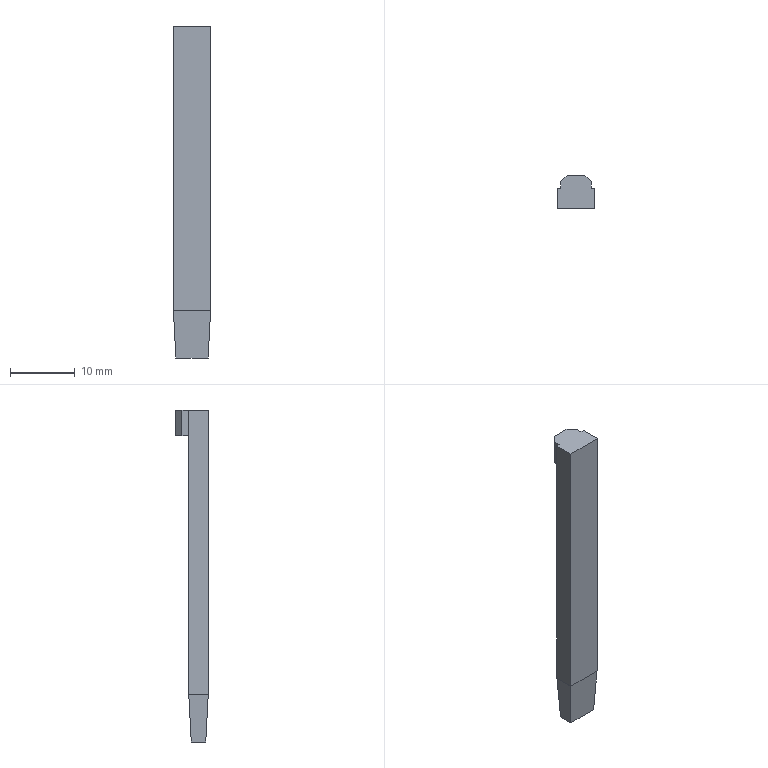Part | Creo | 1 solid | 21 faces | box 5.838 x 5.102 x 51.155 mm | volume 930.54 mm3 | plane 21
STEP:
#1=CARTESIAN_POINT('',(0.,0.,0.));
#2=DIRECTION('',(0.,0.,1.));
#3=DIRECTION('',(1.,0.,0.));
#4=AXIS2_PLACEMENT_3D('',#1,#2,#3);
#5=CARTESIAN_POINT('',(12.137,6.97,42.091));
#6=VERTEX_POINT('',#5);
#7=CARTESIAN_POINT('',(12.137,10.072,42.091));
#8=VERTEX_POINT('',#7);
#9=CARTESIAN_POINT('',(12.137,6.97,42.091));
#10=DIRECTION('',(0.,1.,0.));
#11=VECTOR('',#10,3.102);
#12=LINE('',#9,#11);
#13=EDGE_CURVE('',#6,#8,#12,.T.);
#14=ORIENTED_EDGE('',*,*,#13,.T.);
#15=CARTESIAN_POINT('',(6.299,10.072,42.091));
#16=VERTEX_POINT('',#15);
#17=CARTESIAN_POINT('',(12.137,10.072,42.091));
#18=DIRECTION('',(-1.,0.,0.));
#19=VECTOR('',#18,5.838);
#20=LINE('',#17,#19);
#21=EDGE_CURVE('',#8,#16,#20,.T.);
#22=ORIENTED_EDGE('',*,*,#21,.T.);
#23=CARTESIAN_POINT('',(6.299,6.97,42.091));
#24=VERTEX_POINT('',#23);
#25=CARTESIAN_POINT('',(6.299,10.072,42.091));
#26=DIRECTION('',(0.,-1.,0.));
#27=VECTOR('',#26,3.102);
#28=LINE('',#25,#27);
#29=EDGE_CURVE('',#16,#24,#28,.T.);
#30=ORIENTED_EDGE('',*,*,#29,.T.);
#31=CARTESIAN_POINT('',(6.299,6.97,42.091));
#32=DIRECTION('',(1.,0.,0.));
#33=VECTOR('',#32,5.838);
#34=LINE('',#31,#33);
#35=EDGE_CURVE('',#24,#6,#34,.T.);
#36=ORIENTED_EDGE('',*,*,#35,.T.);
#37=EDGE_LOOP('',(#14,#22,#30,#36));
#38=FACE_OUTER_BOUND('',#37,.F.);
#39=CARTESIAN_POINT('',(12.087,7.02,42.091));
#40=VERTEX_POINT('',#39);
#41=CARTESIAN_POINT('',(12.087,10.022,42.091));
#42=VERTEX_POINT('',#41);
#43=CARTESIAN_POINT('',(12.087,7.02,42.091));
#44=DIRECTION('',(0.,1.,0.));
#45=VECTOR('',#44,3.002);
#46=LINE('',#43,#45);
#47=EDGE_CURVE('',#40,#42,#46,.T.);
#48=ORIENTED_EDGE('',*,*,#47,.F.);
#49=CARTESIAN_POINT('',(6.349,7.02,42.091));
#50=VERTEX_POINT('',#49);
#51=CARTESIAN_POINT('',(6.349,7.02,42.091));
#52=DIRECTION('',(1.,0.,0.));
#53=VECTOR('',#52,5.738);
#54=LINE('',#51,#53);
#55=EDGE_CURVE('',#50,#40,#54,.T.);
#56=ORIENTED_EDGE('',*,*,#55,.F.);
#57=CARTESIAN_POINT('',(6.349,10.022,42.091));
#58=VERTEX_POINT('',#57);
#59=CARTESIAN_POINT('',(6.349,10.022,42.091));
#60=DIRECTION('',(0.,-1.,0.));
#61=VECTOR('',#60,3.002);
#62=LINE('',#59,#61);
#63=EDGE_CURVE('',#58,#50,#62,.T.);
#64=ORIENTED_EDGE('',*,*,#63,.F.);
#65=CARTESIAN_POINT('',(6.349,10.022,42.091));
#66=DIRECTION('',(1.,0.,0.));
#67=VECTOR('',#66,5.738);
#68=LINE('',#65,#67);
#69=EDGE_CURVE('',#58,#42,#68,.T.);
#70=ORIENTED_EDGE('',*,*,#69,.T.);
#71=EDGE_LOOP('',(#48,#56,#64,#70));
#72=FACE_BOUND('',#71,.F.);
#73=CARTESIAN_POINT('',(12.087,10.022,42.091));
#74=DIRECTION('',(0.,0.,1.));
#75=DIRECTION('',(1.,0.,0.));
#76=AXIS2_PLACEMENT_3D('',#73,#74,#75);
#77=PLANE('',#76);
#78=ADVANCED_FACE('',(#38,#72),#77,.F.);
#79=CARTESIAN_POINT('',(12.137,6.97,85.91));
#80=VERTEX_POINT('',#79);
#81=CARTESIAN_POINT('',(12.137,6.97,85.91));
#82=DIRECTION('',(0.,0.,-1.));
#83=VECTOR('',#82,43.819);
#84=LINE('',#81,#83);
#85=EDGE_CURVE('',#80,#6,#84,.T.);
#86=ORIENTED_EDGE('',*,*,#85,.F.);
#87=CARTESIAN_POINT('',(12.137,10.072,85.91));
#88=VERTEX_POINT('',#87);
#89=CARTESIAN_POINT('',(12.137,6.97,85.91));
#90=DIRECTION('',(0.,1.,0.));
#91=VECTOR('',#90,3.102);
#92=LINE('',#89,#91);
#93=EDGE_CURVE('',#80,#88,#92,.T.);
#94=ORIENTED_EDGE('',*,*,#93,.T.);
#95=CARTESIAN_POINT('',(12.137,10.072,85.91));
#96=DIRECTION('',(0.,0.,-1.));
#97=VECTOR('',#96,43.819);
#98=LINE('',#95,#97);
#99=EDGE_CURVE('',#88,#8,#98,.T.);
#100=ORIENTED_EDGE('',*,*,#99,.T.);
#101=ORIENTED_EDGE('',*,*,#13,.F.);
#102=EDGE_LOOP('',(#86,#94,#100,#101));
#103=FACE_OUTER_BOUND('',#102,.F.);
#104=CARTESIAN_POINT('',(12.137,8.521,33.755));
#105=DIRECTION('',(1.,0.,0.));
#106=DIRECTION('',(0.,0.,-1.));
#107=AXIS2_PLACEMENT_3D('',#104,#105,#106);
#108=PLANE('',#107);
#109=ADVANCED_FACE('',(#103),#108,.T.);
#110=CARTESIAN_POINT('',(6.299,6.97,85.91));
#111=VERTEX_POINT('',#110);
#112=CARTESIAN_POINT('',(6.299,6.97,85.91));
#113=DIRECTION('',(0.,0.,-1.));
#114=VECTOR('',#113,43.819);
#115=LINE('',#112,#114);
#116=EDGE_CURVE('',#111,#24,#115,.T.);
#117=ORIENTED_EDGE('',*,*,#116,.F.);
#118=CARTESIAN_POINT('',(6.299,6.97,85.91));
#119=DIRECTION('',(1.,0.,0.));
#120=VECTOR('',#119,5.838);
#121=LINE('',#118,#120);
#122=EDGE_CURVE('',#111,#80,#121,.T.);
#123=ORIENTED_EDGE('',*,*,#122,.T.);
#124=ORIENTED_EDGE('',*,*,#85,.T.);
#125=ORIENTED_EDGE('',*,*,#35,.F.);
#126=EDGE_LOOP('',(#117,#123,#124,#125));
#127=FACE_OUTER_BOUND('',#126,.F.);
#128=CARTESIAN_POINT('',(9.218,6.97,33.755));
#129=DIRECTION('',(0.,-1.,0.));
#130=DIRECTION('',(0.,0.,-1.));
#131=AXIS2_PLACEMENT_3D('',#128,#129,#130);
#132=PLANE('',#131);
#133=ADVANCED_FACE('',(#127),#132,.T.);
#134=CARTESIAN_POINT('',(6.299,10.072,85.91));
#135=VERTEX_POINT('',#134);
#136=CARTESIAN_POINT('',(6.299,10.072,85.91));
#137=DIRECTION('',(0.,0.,-1.));
#138=VECTOR('',#137,43.819);
#139=LINE('',#136,#138);
#140=EDGE_CURVE('',#135,#16,#139,.T.);
#141=ORIENTED_EDGE('',*,*,#140,.F.);
#142=CARTESIAN_POINT('',(6.299,10.072,85.91));
#143=DIRECTION('',(0.,-1.,0.));
#144=VECTOR('',#143,3.102);
#145=LINE('',#142,#144);
#146=EDGE_CURVE('',#135,#111,#145,.T.);
#147=ORIENTED_EDGE('',*,*,#146,.T.);
#148=ORIENTED_EDGE('',*,*,#116,.T.);
#149=ORIENTED_EDGE('',*,*,#29,.F.);
#150=EDGE_LOOP('',(#141,#147,#148,#149));
#151=FACE_OUTER_BOUND('',#150,.F.);
#152=CARTESIAN_POINT('',(6.299,8.521,33.755));
#153=DIRECTION('',(-1.,0.,0.));
#154=DIRECTION('',(0.,0.,1.));
#155=AXIS2_PLACEMENT_3D('',#152,#153,#154);
#156=PLANE('',#155);
#157=ADVANCED_FACE('',(#151),#156,.T.);
#158=ORIENTED_EDGE('',*,*,#99,.F.);
#159=CARTESIAN_POINT('',(11.587,10.072,85.91));
#160=VERTEX_POINT('',#159);
#161=CARTESIAN_POINT('',(12.137,10.072,85.91));
#162=DIRECTION('',(-1.,0.,0.));
#163=VECTOR('',#162,0.55);
#164=LINE('',#161,#163);
#165=EDGE_CURVE('',#88,#160,#164,.T.);
#166=ORIENTED_EDGE('',*,*,#165,.T.);
#167=CARTESIAN_POINT('',(11.587,10.072,81.91));
#168=VERTEX_POINT('',#167);
#169=CARTESIAN_POINT('',(11.587,10.072,81.91));
#170=DIRECTION('',(0.,0.,1.));
#171=VECTOR('',#170,4.);
#172=LINE('',#169,#171);
#173=EDGE_CURVE('',#168,#160,#172,.T.);
#174=ORIENTED_EDGE('',*,*,#173,.F.);
#175=CARTESIAN_POINT('',(6.849,10.072,81.91));
#176=VERTEX_POINT('',#175);
#177=CARTESIAN_POINT('',(6.849,10.072,81.91));
#178=DIRECTION('',(1.,0.,0.));
#179=VECTOR('',#178,4.738);
#180=LINE('',#177,#179);
#181=EDGE_CURVE('',#176,#168,#180,.T.);
#182=ORIENTED_EDGE('',*,*,#181,.F.);
#183=CARTESIAN_POINT('',(6.849,10.072,85.91));
#184=VERTEX_POINT('',#183);
#185=CARTESIAN_POINT('',(6.849,10.072,85.91));
#186=DIRECTION('',(0.,0.,-1.));
#187=VECTOR('',#186,4.);
#188=LINE('',#185,#187);
#189=EDGE_CURVE('',#184,#176,#188,.T.);
#190=ORIENTED_EDGE('',*,*,#189,.F.);
#191=CARTESIAN_POINT('',(6.849,10.072,85.91));
#192=DIRECTION('',(-1.,0.,0.));
#193=VECTOR('',#192,0.55);
#194=LINE('',#191,#193);
#195=EDGE_CURVE('',#184,#135,#194,.T.);
#196=ORIENTED_EDGE('',*,*,#195,.T.);
#197=ORIENTED_EDGE('',*,*,#140,.T.);
#198=ORIENTED_EDGE('',*,*,#21,.F.);
#199=EDGE_LOOP('',(#158,#166,#174,#182,#190,#196,#197,#198));
#200=FACE_OUTER_BOUND('',#199,.F.);
#201=CARTESIAN_POINT('',(9.218,10.072,33.755));
#202=DIRECTION('',(0.,1.,0.));
#203=DIRECTION('',(0.,0.,1.));
#204=AXIS2_PLACEMENT_3D('',#201,#202,#203);
#205=PLANE('',#204);
#206=ADVANCED_FACE('',(#200),#205,.T.);
#207=CARTESIAN_POINT('',(11.587,11.072,85.91));
#208=VERTEX_POINT('',#207);
#209=CARTESIAN_POINT('',(11.587,10.072,85.91));
#210=DIRECTION('',(0.,1.,0.));
#211=VECTOR('',#210,1.);
#212=LINE('',#209,#211);
#213=EDGE_CURVE('',#160,#208,#212,.T.);
#214=ORIENTED_EDGE('',*,*,#213,.F.);
#215=ORIENTED_EDGE('',*,*,#165,.F.);
#216=ORIENTED_EDGE('',*,*,#93,.F.);
#217=ORIENTED_EDGE('',*,*,#122,.F.);
#218=ORIENTED_EDGE('',*,*,#146,.F.);
#219=ORIENTED_EDGE('',*,*,#195,.F.);
#220=CARTESIAN_POINT('',(6.849,11.072,85.91));
#221=VERTEX_POINT('',#220);
#222=CARTESIAN_POINT('',(6.849,11.072,85.91));
#223=DIRECTION('',(0.,-1.,0.));
#224=VECTOR('',#223,1.);
#225=LINE('',#222,#224);
#226=EDGE_CURVE('',#221,#184,#225,.T.);
#227=ORIENTED_EDGE('',*,*,#226,.F.);
#228=CARTESIAN_POINT('',(7.849,12.072,85.91));
#229=VERTEX_POINT('',#228);
#230=CARTESIAN_POINT('',(7.849,12.072,85.91));
#231=DIRECTION('',(-0.7071,-0.7071,0.));
#232=VECTOR('',#231,1.414);
#233=LINE('',#230,#232);
#234=EDGE_CURVE('',#229,#221,#233,.T.);
#235=ORIENTED_EDGE('',*,*,#234,.F.);
#236=CARTESIAN_POINT('',(10.587,12.072,85.91));
#237=VERTEX_POINT('',#236);
#238=CARTESIAN_POINT('',(10.587,12.072,85.91));
#239=DIRECTION('',(-1.,0.,0.));
#240=VECTOR('',#239,2.738);
#241=LINE('',#238,#240);
#242=EDGE_CURVE('',#237,#229,#241,.T.);
#243=ORIENTED_EDGE('',*,*,#242,.F.);
#244=CARTESIAN_POINT('',(11.587,11.072,85.91));
#245=DIRECTION('',(-0.7071,0.7071,0.));
#246=VECTOR('',#245,1.414);
#247=LINE('',#244,#246);
#248=EDGE_CURVE('',#208,#237,#247,.T.);
#249=ORIENTED_EDGE('',*,*,#248,.F.);
#250=EDGE_LOOP('',(#214,#215,#216,#217,#218,#219,#227,#235,#243,#249));
#251=FACE_OUTER_BOUND('',#250,.F.);
#252=CARTESIAN_POINT('',(62.144,-0.4125,85.91));
#253=DIRECTION('',(0.,0.,1.));
#254=DIRECTION('',(0.,1.,0.));
#255=AXIS2_PLACEMENT_3D('',#252,#253,#254);
#256=PLANE('',#255);
#257=ADVANCED_FACE('',(#251),#256,.T.);
#258=CARTESIAN_POINT('',(11.587,11.072,81.91));
#259=VERTEX_POINT('',#258);
#260=CARTESIAN_POINT('',(11.587,11.072,81.91));
#261=DIRECTION('',(0.,-1.,0.));
#262=VECTOR('',#261,1.);
#263=LINE('',#260,#262);
#264=EDGE_CURVE('',#259,#168,#263,.T.);
#265=ORIENTED_EDGE('',*,*,#264,.T.);
#266=ORIENTED_EDGE('',*,*,#173,.T.);
#267=ORIENTED_EDGE('',*,*,#213,.T.);
#268=CARTESIAN_POINT('',(11.587,11.072,85.91));
#269=DIRECTION('',(0.,0.,-1.));
#270=VECTOR('',#269,4.);
#271=LINE('',#268,#270);
#272=EDGE_CURVE('',#208,#259,#271,.T.);
#273=ORIENTED_EDGE('',*,*,#272,.T.);
#274=EDGE_LOOP('',(#265,#266,#267,#273));
#275=FACE_OUTER_BOUND('',#274,.F.);
#276=CARTESIAN_POINT('',(11.587,10.522,81.91));
#277=DIRECTION('',(1.,0.,0.));
#278=DIRECTION('',(0.,0.,-1.));
#279=AXIS2_PLACEMENT_3D('',#276,#277,#278);
#280=PLANE('',#279);
#281=ADVANCED_FACE('',(#275),#280,.T.);
#282=CARTESIAN_POINT('',(7.849,12.072,81.91));
#283=VERTEX_POINT('',#282);
#284=CARTESIAN_POINT('',(10.587,12.072,81.91));
#285=VERTEX_POINT('',#284);
#286=CARTESIAN_POINT('',(7.849,12.072,81.91));
#287=DIRECTION('',(1.,0.,0.));
#288=VECTOR('',#287,2.738);
#289=LINE('',#286,#288);
#290=EDGE_CURVE('',#283,#285,#289,.T.);
#291=ORIENTED_EDGE('',*,*,#290,.F.);
#292=CARTESIAN_POINT('',(6.849,11.072,81.91));
#293=VERTEX_POINT('',#292);
#294=CARTESIAN_POINT('',(6.849,11.072,81.91));
#295=DIRECTION('',(0.7071,0.7071,0.));
#296=VECTOR('',#295,1.414);
#297=LINE('',#294,#296);
#298=EDGE_CURVE('',#293,#283,#297,.T.);
#299=ORIENTED_EDGE('',*,*,#298,.F.);
#300=CARTESIAN_POINT('',(6.849,10.072,81.91));
#301=DIRECTION('',(0.,1.,0.));
#302=VECTOR('',#301,1.);
#303=LINE('',#300,#302);
#304=EDGE_CURVE('',#176,#293,#303,.T.);
#305=ORIENTED_EDGE('',*,*,#304,.F.);
#306=ORIENTED_EDGE('',*,*,#181,.T.);
#307=ORIENTED_EDGE('',*,*,#264,.F.);
#308=CARTESIAN_POINT('',(10.587,12.072,81.91));
#309=DIRECTION('',(0.7071,-0.7071,0.));
#310=VECTOR('',#309,1.414);
#311=LINE('',#308,#310);
#312=EDGE_CURVE('',#285,#259,#311,.T.);
#313=ORIENTED_EDGE('',*,*,#312,.F.);
#314=EDGE_LOOP('',(#291,#299,#305,#306,#307,#313));
#315=FACE_OUTER_BOUND('',#314,.F.);
#316=CARTESIAN_POINT('',(9.218,10.522,81.91));
#317=DIRECTION('',(0.,0.,-1.));
#318=DIRECTION('',(-1.,0.,0.));
#319=AXIS2_PLACEMENT_3D('',#316,#317,#318);
#320=PLANE('',#319);
#321=ADVANCED_FACE('',(#315),#320,.T.);
#322=ORIENTED_EDGE('',*,*,#242,.T.);
#323=CARTESIAN_POINT('',(7.849,12.072,85.91));
#324=DIRECTION('',(0.,0.,-1.));
#325=VECTOR('',#324,4.);
#326=LINE('',#323,#325);
#327=EDGE_CURVE('',#229,#283,#326,.T.);
#328=ORIENTED_EDGE('',*,*,#327,.T.);
#329=ORIENTED_EDGE('',*,*,#290,.T.);
#330=CARTESIAN_POINT('',(10.587,12.072,81.91));
#331=DIRECTION('',(0.,0.,1.));
#332=VECTOR('',#331,4.);
#333=LINE('',#330,#332);
#334=EDGE_CURVE('',#285,#237,#333,.T.);
#335=ORIENTED_EDGE('',*,*,#334,.T.);
#336=EDGE_LOOP('',(#322,#328,#329,#335));
#337=FACE_OUTER_BOUND('',#336,.F.);
#338=CARTESIAN_POINT('',(9.218,12.072,81.91));
#339=DIRECTION('',(0.,1.,0.));
#340=DIRECTION('',(0.,0.,1.));
#341=AXIS2_PLACEMENT_3D('',#338,#339,#340);
#342=PLANE('',#341);
#343=ADVANCED_FACE('',(#337),#342,.T.);
#344=ORIENTED_EDGE('',*,*,#298,.T.);
#345=ORIENTED_EDGE('',*,*,#327,.F.);
#346=ORIENTED_EDGE('',*,*,#234,.T.);
#347=CARTESIAN_POINT('',(6.849,11.072,81.91));
#348=DIRECTION('',(0.,0.,1.));
#349=VECTOR('',#348,4.);
#350=LINE('',#347,#349);
#351=EDGE_CURVE('',#293,#221,#350,.T.);
#352=ORIENTED_EDGE('',*,*,#351,.F.);
#353=EDGE_LOOP('',(#344,#345,#346,#352));
#354=FACE_OUTER_BOUND('',#353,.F.);
#355=CARTESIAN_POINT('',(7.849,12.072,81.91));
#356=DIRECTION('',(0.7071,-0.7071,0.));
#357=DIRECTION('',(0.,0.,1.));
#358=AXIS2_PLACEMENT_3D('',#355,#356,#357);
#359=PLANE('',#358);
#360=ADVANCED_FACE('',(#354),#359,.F.);
#361=ORIENTED_EDGE('',*,*,#226,.T.);
#362=ORIENTED_EDGE('',*,*,#189,.T.);
#363=ORIENTED_EDGE('',*,*,#304,.T.);
#364=ORIENTED_EDGE('',*,*,#351,.T.);
#365=EDGE_LOOP('',(#361,#362,#363,#364));
#366=FACE_OUTER_BOUND('',#365,.F.);
#367=CARTESIAN_POINT('',(6.849,10.522,81.91));
#368=DIRECTION('',(-1.,0.,0.));
#369=DIRECTION('',(0.,0.,1.));
#370=AXIS2_PLACEMENT_3D('',#367,#368,#369);
#371=PLANE('',#370);
#372=ADVANCED_FACE('',(#366),#371,.T.);
#373=ORIENTED_EDGE('',*,*,#312,.T.);
#374=ORIENTED_EDGE('',*,*,#272,.F.);
#375=ORIENTED_EDGE('',*,*,#248,.T.);
#376=ORIENTED_EDGE('',*,*,#334,.F.);
#377=EDGE_LOOP('',(#373,#374,#375,#376));
#378=FACE_OUTER_BOUND('',#377,.F.);
#379=CARTESIAN_POINT('',(11.587,11.072,81.91));
#380=DIRECTION('',(-0.7071,-0.7071,0.));
#381=DIRECTION('',(0.,0.,1.));
#382=AXIS2_PLACEMENT_3D('',#379,#380,#381);
#383=PLANE('',#382);
#384=ADVANCED_FACE('',(#378),#383,.F.);
#385=CARTESIAN_POINT('',(11.703,9.637,34.755));
#386=VERTEX_POINT('',#385);
#387=CARTESIAN_POINT('',(12.087,10.022,42.091));
#388=DIRECTION('',(-0.05226,-0.05226,-0.9973));
#389=VECTOR('',#388,7.357);
#390=LINE('',#387,#389);
#391=EDGE_CURVE('',#42,#386,#390,.T.);
#392=ORIENTED_EDGE('',*,*,#391,.T.);
#393=CARTESIAN_POINT('',(11.703,7.404,34.755));
#394=VERTEX_POINT('',#393);
#395=CARTESIAN_POINT('',(11.703,9.637,34.755));
#396=DIRECTION('',(0.,-1.,0.));
#397=VECTOR('',#396,2.233);
#398=LINE('',#395,#397);
#399=EDGE_CURVE('',#386,#394,#398,.T.);
#400=ORIENTED_EDGE('',*,*,#399,.T.);
#401=CARTESIAN_POINT('',(12.087,7.02,42.091));
#402=DIRECTION('',(-0.05226,0.05226,-0.9973));
#403=VECTOR('',#402,7.357);
#404=LINE('',#401,#403);
#405=EDGE_CURVE('',#40,#394,#404,.T.);
#406=ORIENTED_EDGE('',*,*,#405,.F.);
#407=ORIENTED_EDGE('',*,*,#47,.T.);
#408=EDGE_LOOP('',(#392,#400,#406,#407));
#409=FACE_OUTER_BOUND('',#408,.F.);
#410=CARTESIAN_POINT('',(11.982,12.632,40.081));
#411=DIRECTION('',(0.9986,0.,-0.05234));
#412=DIRECTION('',(0.,1.,0.));
#413=AXIS2_PLACEMENT_3D('',#410,#411,#412);
#414=PLANE('',#413);
#415=ADVANCED_FACE('',(#409),#414,.T.);
#416=CARTESIAN_POINT('',(7.459,9.64,34.794));
#417=VERTEX_POINT('',#416);
#418=CARTESIAN_POINT('',(10.977,9.64,34.794));
#419=VERTEX_POINT('',#418);
#420=CARTESIAN_POINT('',(7.459,9.64,34.794));
#421=DIRECTION('',(1.,0.,0.));
#422=VECTOR('',#421,3.517);
#423=LINE('',#420,#422);
#424=EDGE_CURVE('',#417,#419,#423,.T.);
#425=ORIENTED_EDGE('',*,*,#424,.T.);
#426=CARTESIAN_POINT('',(10.977,9.637,34.755));
#427=VERTEX_POINT('',#426);
#428=CARTESIAN_POINT('',(10.977,9.64,34.794));
#429=DIRECTION('',(0.,-0.05234,-0.9986));
#430=VECTOR('',#429,0.04005);
#431=LINE('',#428,#430);
#432=EDGE_CURVE('',#419,#427,#431,.T.);
#433=ORIENTED_EDGE('',*,*,#432,.T.);
#434=CARTESIAN_POINT('',(10.977,9.637,34.755));
#435=DIRECTION('',(1.,0.,0.));
#436=VECTOR('',#435,0.7259);
#437=LINE('',#434,#436);
#438=EDGE_CURVE('',#427,#386,#437,.T.);
#439=ORIENTED_EDGE('',*,*,#438,.T.);
#440=ORIENTED_EDGE('',*,*,#391,.F.);
#441=ORIENTED_EDGE('',*,*,#69,.F.);
#442=CARTESIAN_POINT('',(6.733,9.637,34.755));
#443=VERTEX_POINT('',#442);
#444=CARTESIAN_POINT('',(6.349,10.022,42.091));
#445=DIRECTION('',(0.05226,-0.05226,-0.9973));
#446=VECTOR('',#445,7.357);
#447=LINE('',#444,#446);
#448=EDGE_CURVE('',#58,#443,#447,.T.);
#449=ORIENTED_EDGE('',*,*,#448,.T.);
#450=CARTESIAN_POINT('',(7.459,9.637,34.755));
#451=VERTEX_POINT('',#450);
#452=CARTESIAN_POINT('',(6.733,9.637,34.755));
#453=DIRECTION('',(1.,0.,0.));
#454=VECTOR('',#453,0.7259);
#455=LINE('',#452,#454);
#456=EDGE_CURVE('',#443,#451,#455,.T.);
#457=ORIENTED_EDGE('',*,*,#456,.T.);
#458=CARTESIAN_POINT('',(7.459,9.637,34.755));
#459=DIRECTION('',(0.,0.05234,0.9986));
#460=VECTOR('',#459,0.04005);
#461=LINE('',#458,#460);
#462=EDGE_CURVE('',#451,#417,#461,.T.);
#463=ORIENTED_EDGE('',*,*,#462,.T.);
#464=EDGE_LOOP('',(#425,#433,#439,#440,#441,#449,#457,#463));
#465=FACE_OUTER_BOUND('',#464,.F.);
#466=CARTESIAN_POINT('',(14.591,9.637,34.755));
#467=DIRECTION('',(0.,-0.9986,0.05234));
#468=DIRECTION('',(-1.,0.,0.));
#469=AXIS2_PLACEMENT_3D('',#466,#467,#468);
#470=PLANE('',#469);
#471=ADVANCED_FACE('',(#465),#470,.F.);
#472=CARTESIAN_POINT('',(10.977,8.24,34.794));
#473=VERTEX_POINT('',#472);
#474=CARTESIAN_POINT('',(10.977,9.64,34.794));
#475=DIRECTION('',(0.,-1.,0.));
#476=VECTOR('',#475,1.399);
#477=LINE('',#474,#476);
#478=EDGE_CURVE('',#419,#473,#477,.T.);
#479=ORIENTED_EDGE('',*,*,#478,.F.);
#480=ORIENTED_EDGE('',*,*,#424,.F.);
#481=CARTESIAN_POINT('',(7.459,8.24,34.794));
#482=VERTEX_POINT('',#481);
#483=CARTESIAN_POINT('',(7.459,8.24,34.794));
#484=DIRECTION('',(0.,1.,0.));
#485=VECTOR('',#484,1.399);
#486=LINE('',#483,#485);
#487=EDGE_CURVE('',#482,#417,#486,.T.);
#488=ORIENTED_EDGE('',*,*,#487,.F.);
#489=CARTESIAN_POINT('',(10.977,8.24,34.794));
#490=DIRECTION('',(-1.,0.,0.));
#491=VECTOR('',#490,3.517);
#492=LINE('',#489,#491);
#493=EDGE_CURVE('',#473,#482,#492,.T.);
#494=ORIENTED_EDGE('',*,*,#493,.F.);
#495=EDGE_LOOP('',(#479,#480,#488,#494));
#496=FACE_OUTER_BOUND('',#495,.F.);
#497=CARTESIAN_POINT('',(-0.07825,-88.35,34.794));
#498=DIRECTION('',(0.,0.,-1.));
#499=DIRECTION('',(0.,-1.,0.));
#500=AXIS2_PLACEMENT_3D('',#497,#498,#499);
#501=PLANE('',#500);
#502=ADVANCED_FACE('',(#496),#501,.T.);
#503=CARTESIAN_POINT('',(10.977,8.24,34.755));
#504=VERTEX_POINT('',#503);
#505=CARTESIAN_POINT('',(10.977,8.24,34.755));
#506=DIRECTION('',(0.,1.,0.));
#507=VECTOR('',#506,1.397);
#508=LINE('',#505,#507);
#509=EDGE_CURVE('',#504,#427,#508,.T.);
#510=ORIENTED_EDGE('',*,*,#509,.T.);
#511=ORIENTED_EDGE('',*,*,#432,.F.);
#512=ORIENTED_EDGE('',*,*,#478,.T.);
#513=CARTESIAN_POINT('',(10.977,8.24,34.755));
#514=DIRECTION('',(0.,0.,1.));
#515=VECTOR('',#514,0.04);
#516=LINE('',#513,#515);
#517=EDGE_CURVE('',#504,#473,#516,.T.);
#518=ORIENTED_EDGE('',*,*,#517,.F.);
#519=EDGE_LOOP('',(#510,#511,#512,#518));
#520=FACE_OUTER_BOUND('',#519,.F.);
#521=CARTESIAN_POINT('',(10.977,9.637,34.255));
#522=DIRECTION('',(-1.,0.,0.));
#523=DIRECTION('',(0.,0.,1.));
#524=AXIS2_PLACEMENT_3D('',#521,#522,#523);
#525=PLANE('',#524);
#526=ADVANCED_FACE('',(#520),#525,.T.);
#527=CARTESIAN_POINT('',(7.459,8.24,34.755));
#528=VERTEX_POINT('',#527);
#529=CARTESIAN_POINT('',(7.459,9.637,34.755));
#530=DIRECTION('',(0.,-1.,0.));
#531=VECTOR('',#530,1.397);
#532=LINE('',#529,#531);
#533=EDGE_CURVE('',#451,#528,#532,.T.);
#534=ORIENTED_EDGE('',*,*,#533,.F.);
#535=ORIENTED_EDGE('',*,*,#456,.F.);
#536=CARTESIAN_POINT('',(6.733,7.404,34.755));
#537=VERTEX_POINT('',#536);
#538=CARTESIAN_POINT('',(6.733,7.404,34.755));
#539=DIRECTION('',(0.,1.,0.));
#540=VECTOR('',#539,2.233);
#541=LINE('',#538,#540);
#542=EDGE_CURVE('',#537,#443,#541,.T.);
#543=ORIENTED_EDGE('',*,*,#542,.F.);
#544=CARTESIAN_POINT('',(11.703,7.404,34.755));
#545=DIRECTION('',(-1.,0.,0.));
#546=VECTOR('',#545,4.969);
#547=LINE('',#544,#546);
#548=EDGE_CURVE('',#394,#537,#547,.T.);
#549=ORIENTED_EDGE('',*,*,#548,.F.);
#550=ORIENTED_EDGE('',*,*,#399,.F.);
#551=ORIENTED_EDGE('',*,*,#438,.F.);
#552=ORIENTED_EDGE('',*,*,#509,.F.);
#553=CARTESIAN_POINT('',(7.459,8.24,34.755));
#554=DIRECTION('',(1.,0.,0.));
#555=VECTOR('',#554,3.517);
#556=LINE('',#553,#555);
#557=EDGE_CURVE('',#528,#504,#556,.T.);
#558=ORIENTED_EDGE('',*,*,#557,.F.);
#559=EDGE_LOOP('',(#534,#535,#543,#549,#550,#551,#552,#558));
#560=FACE_OUTER_BOUND('',#559,.F.);
#561=CARTESIAN_POINT('',(-0.07825,-88.35,34.755));
#562=DIRECTION('',(0.,0.,-1.));
#563=DIRECTION('',(0.,-1.,0.));
#564=AXIS2_PLACEMENT_3D('',#561,#562,#563);
#565=PLANE('',#564);
#566=ADVANCED_FACE('',(#560),#565,.T.);
#567=ORIENTED_EDGE('',*,*,#533,.T.);
#568=CARTESIAN_POINT('',(7.459,8.24,34.755));
#569=DIRECTION('',(0.,0.,1.));
#570=VECTOR('',#569,0.04);
#571=LINE('',#568,#570);
#572=EDGE_CURVE('',#528,#482,#571,.T.);
#573=ORIENTED_EDGE('',*,*,#572,.T.);
#574=ORIENTED_EDGE('',*,*,#487,.T.);
#575=ORIENTED_EDGE('',*,*,#462,.F.);
#576=EDGE_LOOP('',(#567,#573,#574,#575));
#577=FACE_OUTER_BOUND('',#576,.F.);
#578=CARTESIAN_POINT('',(7.459,8.13,34.255));
#579=DIRECTION('',(1.,0.,0.));
#580=DIRECTION('',(0.,0.,-1.));
#581=AXIS2_PLACEMENT_3D('',#578,#579,#580);
#582=PLANE('',#581);
#583=ADVANCED_FACE('',(#577),#582,.T.);
#584=ORIENTED_EDGE('',*,*,#557,.T.);
#585=ORIENTED_EDGE('',*,*,#517,.T.);
#586=ORIENTED_EDGE('',*,*,#493,.T.);
#587=ORIENTED_EDGE('',*,*,#572,.F.);
#588=EDGE_LOOP('',(#584,#585,#586,#587));
#589=FACE_OUTER_BOUND('',#588,.F.);
#590=CARTESIAN_POINT('',(-0.07825,8.24,34.255));
#591=DIRECTION('',(0.,1.,0.));
#592=DIRECTION('',(0.,0.,1.));
#593=AXIS2_PLACEMENT_3D('',#590,#591,#592);
#594=PLANE('',#593);
#595=ADVANCED_FACE('',(#589),#594,.T.);
#596=CARTESIAN_POINT('',(6.349,7.02,42.091));
#597=DIRECTION('',(0.05226,0.05226,-0.9973));
#598=VECTOR('',#597,7.357);
#599=LINE('',#596,#598);
#600=EDGE_CURVE('',#50,#537,#599,.T.);
#601=ORIENTED_EDGE('',*,*,#600,.T.);
#602=ORIENTED_EDGE('',*,*,#542,.T.);
#603=ORIENTED_EDGE('',*,*,#448,.F.);
#604=ORIENTED_EDGE('',*,*,#63,.T.);
#605=EDGE_LOOP('',(#601,#602,#603,#604));
#606=FACE_OUTER_BOUND('',#605,.F.);
#607=CARTESIAN_POINT('',(6.454,4.515,40.081));
#608=DIRECTION('',(-0.9986,0.,-0.05234));
#609=DIRECTION('',(0.,-1.,0.));
#610=AXIS2_PLACEMENT_3D('',#607,#608,#609);
#611=PLANE('',#610);
#612=ADVANCED_FACE('',(#606),#611,.T.);
#613=ORIENTED_EDGE('',*,*,#405,.T.);
#614=ORIENTED_EDGE('',*,*,#548,.T.);
#615=ORIENTED_EDGE('',*,*,#600,.F.);
#616=ORIENTED_EDGE('',*,*,#55,.T.);
#617=EDGE_LOOP('',(#613,#614,#615,#616));
#618=FACE_OUTER_BOUND('',#617,.F.);
#619=CARTESIAN_POINT('',(14.591,7.125,40.081));
#620=DIRECTION('',(0.,-0.9986,-0.05234));
#621=DIRECTION('',(1.,0.,0.));
#622=AXIS2_PLACEMENT_3D('',#619,#620,#621);
#623=PLANE('',#622);
#624=ADVANCED_FACE('',(#618),#623,.T.);
#625=CLOSED_SHELL('',(#78,#109,#133,#157,#206,#257,#281,#321,#343,#360,#372,#384,#415,#471,#502,#526,#566,#583,#595,#612,#624));
#626=MANIFOLD_SOLID_BREP('',#625);
#627=(LENGTH_UNIT()NAMED_UNIT(*)SI_UNIT(.MILLI.,.METRE.));
#628=UNCERTAINTY_MEASURE_WITH_UNIT(LENGTH_MEASURE(0.005174),#627,'','');
#629=(NAMED_UNIT(*)PLANE_ANGLE_UNIT()SI_UNIT($,.RADIAN.));
#630=PLANE_ANGLE_MEASURE_WITH_UNIT(PLANE_ANGLE_MEASURE(0.01745),#629);
#631=(CONVERSION_BASED_UNIT('DEGREE',#630)NAMED_UNIT(*)PLANE_ANGLE_UNIT());
#632=(NAMED_UNIT(*)SI_UNIT($,.STERADIAN.)SOLID_ANGLE_UNIT());
#633=(GEOMETRIC_REPRESENTATION_CONTEXT(3)GLOBAL_UNCERTAINTY_ASSIGNED_CONTEXT((#628))GLOBAL_UNIT_ASSIGNED_CONTEXT((#627,#631,#632))REPRESENTATION_CONTEXT('',''));
#634=ADVANCED_BREP_SHAPE_REPRESENTATION('',(#4,#626),#633);